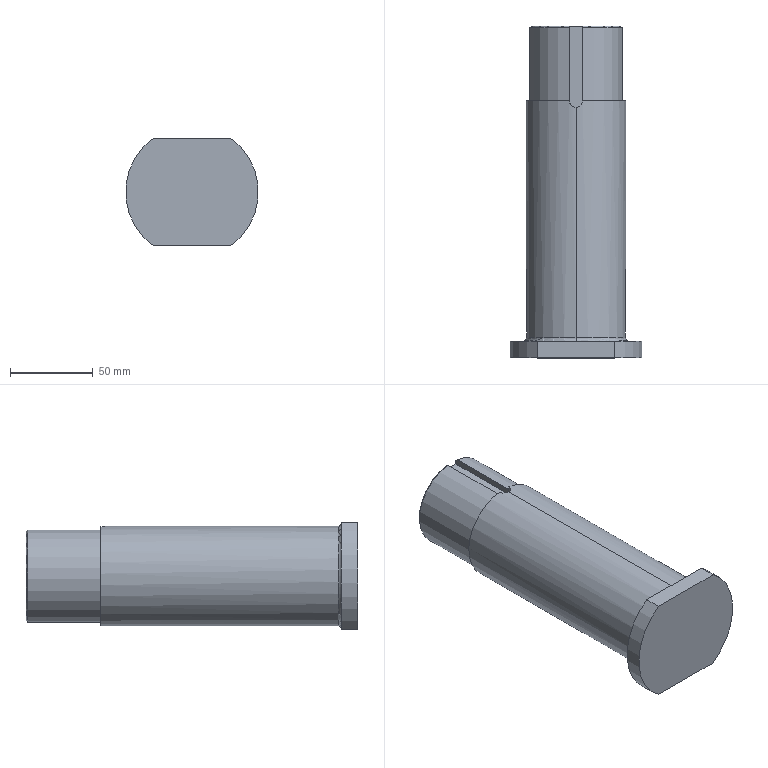Part | SolidWorks | features Fillet 2, ICE 2, Chamfer 1, Revolution 1 | 1 solid | 19 faces | box 80 x 200 x 65 mm | volume 564846 mm3 | plane 9 | cylinder 6 | torus 2 | cone 2 | commonest cylinder face diameters 60 x2 80 x2 8 x1 56 x1
STEP:
#1=CARTESIAN_POINT('',(0.,10.,32.));
#2=VERTEX_POINT('',#1);
#3=CARTESIAN_POINT('',(0.,10.,-32.));
#4=VERTEX_POINT('',#3);
#5=CARTESIAN_POINT('',(0.,10.,0.));
#6=DIRECTION('',(0.,-1.,0.));
#7=DIRECTION('',(0.,0.,-1.));
#8=AXIS2_PLACEMENT_3D('',#5,#6,#7);
#9=CIRCLE('',#8,32.);
#10=EDGE_CURVE('',#2,#4,#9,.T.);
#11=ORIENTED_EDGE('',*,*,#10,.F.);
#12=CARTESIAN_POINT('',(0.,12.,30.));
#13=VERTEX_POINT('',#12);
#14=CARTESIAN_POINT('',(0.,12.,32.));
#15=DIRECTION('',(1.,0.,0.));
#16=DIRECTION('',(0.,0.,-1.));
#17=AXIS2_PLACEMENT_3D('',#14,#15,#16);
#18=CIRCLE('',#17,2.);
#19=EDGE_CURVE('',#2,#13,#18,.T.);
#20=ORIENTED_EDGE('',*,*,#19,.T.);
#21=CARTESIAN_POINT('',(0.,12.,-30.));
#22=VERTEX_POINT('',#21);
#23=CARTESIAN_POINT('',(0.,12.,0.));
#24=DIRECTION('',(0.,1.,0.));
#25=DIRECTION('',(0.,0.,-1.));
#26=AXIS2_PLACEMENT_3D('',#23,#24,#25);
#27=CIRCLE('',#26,30.);
#28=EDGE_CURVE('',#22,#13,#27,.T.);
#29=ORIENTED_EDGE('',*,*,#28,.F.);
#30=CARTESIAN_POINT('',(0.,12.,-32.));
#31=DIRECTION('',(-1.,0.,0.));
#32=DIRECTION('',(0.,0.,1.));
#33=AXIS2_PLACEMENT_3D('',#30,#31,#32);
#34=CIRCLE('',#33,2.);
#35=EDGE_CURVE('',#4,#22,#34,.T.);
#36=ORIENTED_EDGE('',*,*,#35,.F.);
#37=EDGE_LOOP('',(#11,#20,#29,#36));
#38=FACE_OUTER_BOUND('',#37,.T.);
#39=CARTESIAN_POINT('',(0.,12.,0.));
#40=DIRECTION('',(0.,-1.,0.));
#41=DIRECTION('',(0.,0.,-1.));
#42=AXIS2_PLACEMENT_3D('',#39,#40,#41);
#43=TOROIDAL_SURFACE('',#42,32.,2.);
#44=ADVANCED_FACE('',(#38),#43,.F.);
#45=CARTESIAN_POINT('',(0.,200.,-27.));
#46=VERTEX_POINT('',#45);
#47=CARTESIAN_POINT('',(-4.,200.,26.702));
#48=VERTEX_POINT('',#47);
#49=CARTESIAN_POINT('',(0.,200.,0.));
#50=DIRECTION('',(0.,1.,0.));
#51=DIRECTION('',(0.,0.,-1.));
#52=AXIS2_PLACEMENT_3D('',#49,#50,#51);
#53=CIRCLE('',#52,27.);
#54=EDGE_CURVE('',#46,#48,#53,.T.);
#55=ORIENTED_EDGE('',*,*,#54,.F.);
#56=CARTESIAN_POINT('',(0.,199.,-28.));
#57=VERTEX_POINT('',#56);
#58=CARTESIAN_POINT('',(0.,200.,-27.));
#59=DIRECTION('',(0.,-0.7071,-0.7071));
#60=VECTOR('',#59,1000.);
#61=LINE('',#58,#60);
#62=EDGE_CURVE('',#46,#57,#61,.T.);
#63=ORIENTED_EDGE('',*,*,#62,.T.);
#64=CARTESIAN_POINT('',(-4.,199.,27.713));
#65=VERTEX_POINT('',#64);
#66=CARTESIAN_POINT('',(0.,199.,0.));
#67=DIRECTION('',(0.,-1.,0.));
#68=DIRECTION('',(0.,0.,-1.));
#69=AXIS2_PLACEMENT_3D('',#66,#67,#68);
#70=CIRCLE('',#69,28.);
#71=EDGE_CURVE('',#65,#57,#70,.T.);
#72=ORIENTED_EDGE('',*,*,#71,.F.);
#73=CARTESIAN_POINT('',(-4.,200.,26.702));
#74=CARTESIAN_POINT('',(-4.,199.667,27.039));
#75=CARTESIAN_POINT('',(-4.,199.333,27.376));
#76=CARTESIAN_POINT('',(-4.,199.,27.713));
#77=B_SPLINE_CURVE_WITH_KNOTS('',3,(#73,#74,#75,#76),.UNSPECIFIED.,.F.,.F.,(4,4),(0.,0.001422),.UNSPECIFIED.);
#78=EDGE_CURVE('',#48,#65,#77,.T.);
#79=ORIENTED_EDGE('',*,*,#78,.F.);
#80=EDGE_LOOP('',(#55,#63,#72,#79));
#81=FACE_OUTER_BOUND('',#80,.T.);
#82=CARTESIAN_POINT('',(0.,200.,0.));
#83=DIRECTION('',(0.,-1.,0.));
#84=DIRECTION('',(0.,0.,-1.));
#85=AXIS2_PLACEMENT_3D('',#82,#83,#84);
#86=CONICAL_SURFACE('',#85,27.,0.7854);
#87=ADVANCED_FACE('',(#81),#86,.T.);
#88=CARTESIAN_POINT('',(0.,12.,0.));
#89=DIRECTION('',(0.,1.,0.));
#90=DIRECTION('',(0.,0.,-1.));
#91=AXIS2_PLACEMENT_3D('',#88,#89,#90);
#92=CIRCLE('',#91,30.);
#93=EDGE_CURVE('',#13,#22,#92,.T.);
#94=ORIENTED_EDGE('',*,*,#93,.T.);
#95=CARTESIAN_POINT('',(0.,155.,-30.));
#96=VERTEX_POINT('',#95);
#97=CARTESIAN_POINT('',(0.,0.,-30.));
#98=DIRECTION('',(0.,1.,0.));
#99=VECTOR('',#98,1000.);
#100=LINE('',#97,#99);
#101=EDGE_CURVE('',#22,#96,#100,.T.);
#102=ORIENTED_EDGE('',*,*,#101,.T.);
#103=CARTESIAN_POINT('',(4.,155.,29.732));
#104=VERTEX_POINT('',#103);
#105=CARTESIAN_POINT('',(0.,155.,0.));
#106=DIRECTION('',(0.,1.,0.));
#107=DIRECTION('',(0.,0.,1.));
#108=AXIS2_PLACEMENT_3D('',#105,#106,#107);
#109=CIRCLE('',#108,30.);
#110=EDGE_CURVE('',#104,#96,#109,.T.);
#111=ORIENTED_EDGE('',*,*,#110,.F.);
#112=CARTESIAN_POINT('',(0.,151.,30.));
#113=VERTEX_POINT('',#112);
#114=CARTESIAN_POINT('',(4.,155.,29.732));
#115=CARTESIAN_POINT('',(4.,154.735,29.732));
#116=CARTESIAN_POINT('',(3.974,154.475,29.736));
#117=CARTESIAN_POINT('',(3.872,153.963,29.749));
#118=CARTESIAN_POINT('',(3.795,153.709,29.759));
#119=CARTESIAN_POINT('',(3.594,153.225,29.784));
#120=CARTESIAN_POINT('',(3.471,152.995,29.799));
#121=CARTESIAN_POINT('',(3.181,152.56,29.831));
#122=CARTESIAN_POINT('',(3.012,152.355,29.849));
#123=CARTESIAN_POINT('',(2.643,151.986,29.884));
#124=CARTESIAN_POINT('',(2.442,151.821,29.901));
#125=CARTESIAN_POINT('',(2.004,151.528,29.934));
#126=CARTESIAN_POINT('',(1.772,151.404,29.949));
#127=CARTESIAN_POINT('',(1.29,151.205,29.973));
#128=CARTESIAN_POINT('',(1.038,151.128,29.983));
#129=CARTESIAN_POINT('',(0.5211,151.025,29.997));
#130=CARTESIAN_POINT('',(0.2613,151.,30.));
#131=CARTESIAN_POINT('',(0.,151.,30.));
#132=B_SPLINE_CURVE_WITH_KNOTS('',3,(#114,#115,#116,#117,#118,#119,#120,#121,#122,#123,#124,#125,#126,#127,#128,#129,#130,#131),.UNSPECIFIED.,.F.,.F.,(4,2,2,2,2,2,2,2,4),(0.,0.0007827,0.001565,0.002348,0.003131,0.003913,0.004696,0.005479,0.006261),.UNSPECIFIED.);
#133=EDGE_CURVE('',#104,#113,#132,.T.);
#134=ORIENTED_EDGE('',*,*,#133,.T.);
#135=CARTESIAN_POINT('',(0.,0.,30.));
#136=DIRECTION('',(0.,1.,0.));
#137=VECTOR('',#136,1000.);
#138=LINE('',#135,#137);
#139=EDGE_CURVE('',#13,#113,#138,.T.);
#140=ORIENTED_EDGE('',*,*,#139,.F.);
#141=EDGE_LOOP('',(#94,#102,#111,#134,#140));
#142=FACE_OUTER_BOUND('',#141,.T.);
#143=CARTESIAN_POINT('',(0.,0.,0.));
#144=DIRECTION('',(0.,1.,0.));
#145=DIRECTION('',(0.,0.,1.));
#146=AXIS2_PLACEMENT_3D('',#143,#144,#145);
#147=CYLINDRICAL_SURFACE('',#146,30.);
#148=ADVANCED_FACE('',(#142),#147,.T.);
#149=ORIENTED_EDGE('',*,*,#101,.F.);
#150=ORIENTED_EDGE('',*,*,#28,.T.);
#151=ORIENTED_EDGE('',*,*,#139,.T.);
#152=CARTESIAN_POINT('',(-4.,155.,29.732));
#153=VERTEX_POINT('',#152);
#154=CARTESIAN_POINT('',(0.,151.,30.));
#155=CARTESIAN_POINT('',(-0.261,151.,30.));
#156=CARTESIAN_POINT('',(-0.5262,151.026,29.996));
#157=CARTESIAN_POINT('',(-1.039,151.128,29.983));
#158=CARTESIAN_POINT('',(-1.288,151.204,29.973));
#159=CARTESIAN_POINT('',(-1.773,151.405,29.949));
#160=CARTESIAN_POINT('',(-2.006,151.53,29.934));
#161=CARTESIAN_POINT('',(-2.439,151.819,29.901));
#162=CARTESIAN_POINT('',(-2.641,151.984,29.884));
#163=CARTESIAN_POINT('',(-3.014,152.357,29.849));
#164=CARTESIAN_POINT('',(-3.179,152.559,29.831));
#165=CARTESIAN_POINT('',(-3.469,152.991,29.799));
#166=CARTESIAN_POINT('',(-3.594,153.225,29.784));
#167=CARTESIAN_POINT('',(-3.795,153.709,29.759));
#168=CARTESIAN_POINT('',(-3.871,153.958,29.749));
#169=CARTESIAN_POINT('',(-3.973,154.471,29.736));
#170=CARTESIAN_POINT('',(-4.,154.736,29.732));
#171=CARTESIAN_POINT('',(-4.,155.,29.732));
#172=B_SPLINE_CURVE_WITH_KNOTS('',3,(#154,#155,#156,#157,#158,#159,#160,#161,#162,#163,#164,#165,#166,#167,#168,#169,#170,#171),.UNSPECIFIED.,.F.,.F.,(4,2,2,2,2,2,2,2,4),(0.006261,0.007043,0.007825,0.008607,0.009389,0.01017,0.01095,0.01173,0.01252),.UNSPECIFIED.);
#173=EDGE_CURVE('',#113,#153,#172,.T.);
#174=ORIENTED_EDGE('',*,*,#173,.T.);
#175=CARTESIAN_POINT('',(0.,155.,0.));
#176=DIRECTION('',(0.,1.,0.));
#177=DIRECTION('',(0.,0.,1.));
#178=AXIS2_PLACEMENT_3D('',#175,#176,#177);
#179=CIRCLE('',#178,30.);
#180=EDGE_CURVE('',#96,#153,#179,.T.);
#181=ORIENTED_EDGE('',*,*,#180,.F.);
#182=EDGE_LOOP('',(#149,#150,#151,#174,#181));
#183=FACE_OUTER_BOUND('',#182,.T.);
#184=CARTESIAN_POINT('',(0.,0.,0.));
#185=DIRECTION('',(0.,1.,0.));
#186=DIRECTION('',(0.,0.,1.));
#187=AXIS2_PLACEMENT_3D('',#184,#185,#186);
#188=CYLINDRICAL_SURFACE('',#187,30.);
#189=ADVANCED_FACE('',(#183),#188,.T.);
#190=CARTESIAN_POINT('',(-4.,155.,27.713));
#191=VERTEX_POINT('',#190);
#192=CARTESIAN_POINT('',(-4.,155.,32.501));
#193=DIRECTION('',(0.,0.,-1.));
#194=VECTOR('',#193,1000.);
#195=LINE('',#192,#194);
#196=EDGE_CURVE('',#153,#191,#195,.T.);
#197=ORIENTED_EDGE('',*,*,#196,.T.);
#198=CARTESIAN_POINT('',(4.,155.,27.713));
#199=VERTEX_POINT('',#198);
#200=CARTESIAN_POINT('',(0.,155.,0.));
#201=DIRECTION('',(0.,1.,0.));
#202=DIRECTION('',(0.,0.,1.));
#203=AXIS2_PLACEMENT_3D('',#200,#201,#202);
#204=CIRCLE('',#203,28.);
#205=EDGE_CURVE('',#199,#191,#204,.T.);
#206=ORIENTED_EDGE('',*,*,#205,.F.);
#207=CARTESIAN_POINT('',(4.,155.,32.501));
#208=DIRECTION('',(0.,0.,-1.));
#209=VECTOR('',#208,1000.);
#210=LINE('',#207,#209);
#211=EDGE_CURVE('',#104,#199,#210,.T.);
#212=ORIENTED_EDGE('',*,*,#211,.F.);
#213=ORIENTED_EDGE('',*,*,#110,.T.);
#214=ORIENTED_EDGE('',*,*,#180,.T.);
#215=EDGE_LOOP('',(#197,#206,#212,#213,#214));
#216=FACE_OUTER_BOUND('',#215,.T.);
#217=CARTESIAN_POINT('',(30.,155.,0.));
#218=DIRECTION('',(0.,-1.,0.));
#219=DIRECTION('',(0.,0.,-1.));
#220=AXIS2_PLACEMENT_3D('',#217,#218,#219);
#221=PLANE('',#220);
#222=ADVANCED_FACE('',(#216),#221,.F.);
#223=CARTESIAN_POINT('',(-4.,0.,27.713));
#224=DIRECTION('',(0.,1.,0.));
#225=VECTOR('',#224,1000.);
#226=LINE('',#223,#225);
#227=EDGE_CURVE('',#191,#65,#226,.T.);
#228=ORIENTED_EDGE('',*,*,#227,.T.);
#229=ORIENTED_EDGE('',*,*,#71,.T.);
#230=CARTESIAN_POINT('',(4.,199.,27.713));
#231=VERTEX_POINT('',#230);
#232=CARTESIAN_POINT('',(0.,199.,0.));
#233=DIRECTION('',(0.,-1.,0.));
#234=DIRECTION('',(0.,0.,-1.));
#235=AXIS2_PLACEMENT_3D('',#232,#233,#234);
#236=CIRCLE('',#235,28.);
#237=EDGE_CURVE('',#57,#231,#236,.T.);
#238=ORIENTED_EDGE('',*,*,#237,.T.);
#239=CARTESIAN_POINT('',(4.,0.,27.713));
#240=DIRECTION('',(0.,-1.,0.));
#241=VECTOR('',#240,1000.);
#242=LINE('',#239,#241);
#243=EDGE_CURVE('',#231,#199,#242,.T.);
#244=ORIENTED_EDGE('',*,*,#243,.T.);
#245=ORIENTED_EDGE('',*,*,#205,.T.);
#246=EDGE_LOOP('',(#228,#229,#238,#244,#245));
#247=FACE_OUTER_BOUND('',#246,.T.);
#248=CARTESIAN_POINT('',(0.,0.,0.));
#249=DIRECTION('',(0.,1.,0.));
#250=DIRECTION('',(0.,0.,1.));
#251=AXIS2_PLACEMENT_3D('',#248,#249,#250);
#252=CYLINDRICAL_SURFACE('',#251,28.);
#253=ADVANCED_FACE('',(#247),#252,.T.);
#254=CARTESIAN_POINT('',(4.,200.,24.));
#255=VERTEX_POINT('',#254);
#256=CARTESIAN_POINT('',(4.,200.,26.702));
#257=VERTEX_POINT('',#256);
#258=CARTESIAN_POINT('',(4.,200.,32.501));
#259=DIRECTION('',(0.,0.,1.));
#260=VECTOR('',#259,1000.);
#261=LINE('',#258,#260);
#262=EDGE_CURVE('',#255,#257,#261,.T.);
#263=ORIENTED_EDGE('',*,*,#262,.T.);
#264=CARTESIAN_POINT('',(0.,200.,0.));
#265=DIRECTION('',(0.,1.,0.));
#266=DIRECTION('',(0.,0.,-1.));
#267=AXIS2_PLACEMENT_3D('',#264,#265,#266);
#268=CIRCLE('',#267,27.);
#269=EDGE_CURVE('',#257,#46,#268,.T.);
#270=ORIENTED_EDGE('',*,*,#269,.T.);
#271=ORIENTED_EDGE('',*,*,#54,.T.);
#272=CARTESIAN_POINT('',(-4.,200.,24.));
#273=VERTEX_POINT('',#272);
#274=CARTESIAN_POINT('',(-4.,200.,32.501));
#275=DIRECTION('',(0.,0.,-1.));
#276=VECTOR('',#275,1000.);
#277=LINE('',#274,#276);
#278=EDGE_CURVE('',#48,#273,#277,.T.);
#279=ORIENTED_EDGE('',*,*,#278,.T.);
#280=CARTESIAN_POINT('',(0.,200.,24.));
#281=DIRECTION('',(1.,0.,0.));
#282=VECTOR('',#281,1000.);
#283=LINE('',#280,#282);
#284=EDGE_CURVE('',#273,#255,#283,.T.);
#285=ORIENTED_EDGE('',*,*,#284,.T.);
#286=EDGE_LOOP('',(#263,#270,#271,#279,#285));
#287=FACE_OUTER_BOUND('',#286,.T.);
#288=CARTESIAN_POINT('',(28.,200.,0.));
#289=DIRECTION('',(0.,-1.,0.));
#290=DIRECTION('',(0.,0.,-1.));
#291=AXIS2_PLACEMENT_3D('',#288,#289,#290);
#292=PLANE('',#291);
#293=ADVANCED_FACE('',(#287),#292,.F.);
#294=CARTESIAN_POINT('',(-23.318,0.,-32.5));
#295=VERTEX_POINT('',#294);
#296=CARTESIAN_POINT('',(-23.318,0.,32.5));
#297=VERTEX_POINT('',#296);
#298=CARTESIAN_POINT('',(0.,0.,0.));
#299=DIRECTION('',(0.,1.,0.));
#300=DIRECTION('',(0.,0.,1.));
#301=AXIS2_PLACEMENT_3D('',#298,#299,#300);
#302=CIRCLE('',#301,40.);
#303=EDGE_CURVE('',#295,#297,#302,.T.);
#304=ORIENTED_EDGE('',*,*,#303,.T.);
#305=CARTESIAN_POINT('',(-23.318,10.,32.5));
#306=VERTEX_POINT('',#305);
#307=CARTESIAN_POINT('',(-23.318,0.,32.5));
#308=DIRECTION('',(0.,1.,0.));
#309=VECTOR('',#308,1000.);
#310=LINE('',#307,#309);
#311=EDGE_CURVE('',#297,#306,#310,.T.);
#312=ORIENTED_EDGE('',*,*,#311,.T.);
#313=CARTESIAN_POINT('',(-23.318,10.,-32.5));
#314=VERTEX_POINT('',#313);
#315=CARTESIAN_POINT('',(0.,10.,0.));
#316=DIRECTION('',(0.,1.,0.));
#317=DIRECTION('',(0.,0.,1.));
#318=AXIS2_PLACEMENT_3D('',#315,#316,#317);
#319=CIRCLE('',#318,40.);
#320=EDGE_CURVE('',#314,#306,#319,.T.);
#321=ORIENTED_EDGE('',*,*,#320,.F.);
#322=CARTESIAN_POINT('',(-23.318,0.,-32.5));
#323=DIRECTION('',(0.,-1.,0.));
#324=VECTOR('',#323,1000.);
#325=LINE('',#322,#324);
#326=EDGE_CURVE('',#314,#295,#325,.T.);
#327=ORIENTED_EDGE('',*,*,#326,.T.);
#328=EDGE_LOOP('',(#304,#312,#321,#327));
#329=FACE_OUTER_BOUND('',#328,.T.);
#330=CARTESIAN_POINT('',(0.,0.,0.));
#331=DIRECTION('',(0.,1.,0.));
#332=DIRECTION('',(0.,0.,1.));
#333=AXIS2_PLACEMENT_3D('',#330,#331,#332);
#334=CYLINDRICAL_SURFACE('',#333,40.);
#335=ADVANCED_FACE('',(#329),#334,.T.);
#336=CARTESIAN_POINT('',(23.318,0.,32.5));
#337=VERTEX_POINT('',#336);
#338=CARTESIAN_POINT('',(23.318,0.,-32.5));
#339=VERTEX_POINT('',#338);
#340=CARTESIAN_POINT('',(0.,0.,0.));
#341=DIRECTION('',(0.,1.,0.));
#342=DIRECTION('',(0.,0.,1.));
#343=AXIS2_PLACEMENT_3D('',#340,#341,#342);
#344=CIRCLE('',#343,40.);
#345=EDGE_CURVE('',#337,#339,#344,.T.);
#346=ORIENTED_EDGE('',*,*,#345,.F.);
#347=CARTESIAN_POINT('',(65.,0.,32.5));
#348=DIRECTION('',(1.,0.,0.));
#349=VECTOR('',#348,1000.);
#350=LINE('',#347,#349);
#351=EDGE_CURVE('',#297,#337,#350,.T.);
#352=ORIENTED_EDGE('',*,*,#351,.F.);
#353=ORIENTED_EDGE('',*,*,#303,.F.);
#354=CARTESIAN_POINT('',(65.,0.,-32.5));
#355=DIRECTION('',(-1.,0.,0.));
#356=VECTOR('',#355,1000.);
#357=LINE('',#354,#356);
#358=EDGE_CURVE('',#339,#295,#357,.T.);
#359=ORIENTED_EDGE('',*,*,#358,.F.);
#360=EDGE_LOOP('',(#346,#352,#353,#359));
#361=FACE_OUTER_BOUND('',#360,.T.);
#362=CARTESIAN_POINT('',(0.,0.,0.));
#363=DIRECTION('',(0.,1.,0.));
#364=DIRECTION('',(0.,0.,1.));
#365=AXIS2_PLACEMENT_3D('',#362,#363,#364);
#366=PLANE('',#365);
#367=ADVANCED_FACE('',(#361),#366,.F.);
#368=CARTESIAN_POINT('',(23.318,10.,32.5));
#369=VERTEX_POINT('',#368);
#370=CARTESIAN_POINT('',(23.318,10.,-32.5));
#371=VERTEX_POINT('',#370);
#372=CARTESIAN_POINT('',(0.,10.,0.));
#373=DIRECTION('',(0.,1.,0.));
#374=DIRECTION('',(0.,0.,1.));
#375=AXIS2_PLACEMENT_3D('',#372,#373,#374);
#376=CIRCLE('',#375,40.);
#377=EDGE_CURVE('',#369,#371,#376,.T.);
#378=ORIENTED_EDGE('',*,*,#377,.F.);
#379=CARTESIAN_POINT('',(23.318,0.,32.5));
#380=DIRECTION('',(0.,-1.,0.));
#381=VECTOR('',#380,1000.);
#382=LINE('',#379,#381);
#383=EDGE_CURVE('',#369,#337,#382,.T.);
#384=ORIENTED_EDGE('',*,*,#383,.T.);
#385=ORIENTED_EDGE('',*,*,#345,.T.);
#386=CARTESIAN_POINT('',(23.318,0.,-32.5));
#387=DIRECTION('',(0.,1.,0.));
#388=VECTOR('',#387,1000.);
#389=LINE('',#386,#388);
#390=EDGE_CURVE('',#339,#371,#389,.T.);
#391=ORIENTED_EDGE('',*,*,#390,.T.);
#392=EDGE_LOOP('',(#378,#384,#385,#391));
#393=FACE_OUTER_BOUND('',#392,.T.);
#394=CARTESIAN_POINT('',(0.,0.,0.));
#395=DIRECTION('',(0.,1.,0.));
#396=DIRECTION('',(0.,0.,1.));
#397=AXIS2_PLACEMENT_3D('',#394,#395,#396);
#398=CYLINDRICAL_SURFACE('',#397,40.);
#399=ADVANCED_FACE('',(#393),#398,.T.);
#400=CARTESIAN_POINT('',(0.,10.,0.));
#401=DIRECTION('',(0.,-1.,0.));
#402=DIRECTION('',(0.,0.,-1.));
#403=AXIS2_PLACEMENT_3D('',#400,#401,#402);
#404=CIRCLE('',#403,32.);
#405=EDGE_CURVE('',#4,#2,#404,.T.);
#406=ORIENTED_EDGE('',*,*,#405,.T.);
#407=ORIENTED_EDGE('',*,*,#10,.T.);
#408=EDGE_LOOP('',(#406,#407));
#409=FACE_BOUND('',#408,.T.);
#410=ORIENTED_EDGE('',*,*,#320,.T.);
#411=CARTESIAN_POINT('',(40.,10.,32.5));
#412=DIRECTION('',(1.,0.,0.));
#413=VECTOR('',#412,1000.);
#414=LINE('',#411,#413);
#415=EDGE_CURVE('',#306,#369,#414,.T.);
#416=ORIENTED_EDGE('',*,*,#415,.T.);
#417=ORIENTED_EDGE('',*,*,#377,.T.);
#418=CARTESIAN_POINT('',(40.,10.,-32.5));
#419=DIRECTION('',(-1.,0.,0.));
#420=VECTOR('',#419,1000.);
#421=LINE('',#418,#420);
#422=EDGE_CURVE('',#371,#314,#421,.T.);
#423=ORIENTED_EDGE('',*,*,#422,.T.);
#424=EDGE_LOOP('',(#410,#416,#417,#423));
#425=FACE_OUTER_BOUND('',#424,.T.);
#426=CARTESIAN_POINT('',(40.,10.,0.));
#427=DIRECTION('',(0.,-1.,0.));
#428=DIRECTION('',(0.,0.,-1.));
#429=AXIS2_PLACEMENT_3D('',#426,#427,#428);
#430=PLANE('',#429);
#431=ADVANCED_FACE('',(#409,#425),#430,.F.);
#432=ORIENTED_EDGE('',*,*,#358,.T.);
#433=ORIENTED_EDGE('',*,*,#326,.F.);
#434=ORIENTED_EDGE('',*,*,#422,.F.);
#435=ORIENTED_EDGE('',*,*,#390,.F.);
#436=EDGE_LOOP('',(#432,#433,#434,#435));
#437=FACE_OUTER_BOUND('',#436,.T.);
#438=CARTESIAN_POINT('',(65.,10.,-32.5));
#439=DIRECTION('',(0.,0.,1.));
#440=DIRECTION('',(1.,0.,0.));
#441=AXIS2_PLACEMENT_3D('',#438,#439,#440);
#442=PLANE('',#441);
#443=ADVANCED_FACE('',(#437),#442,.F.);
#444=ORIENTED_EDGE('',*,*,#351,.T.);
#445=ORIENTED_EDGE('',*,*,#383,.F.);
#446=ORIENTED_EDGE('',*,*,#415,.F.);
#447=ORIENTED_EDGE('',*,*,#311,.F.);
#448=EDGE_LOOP('',(#444,#445,#446,#447));
#449=FACE_OUTER_BOUND('',#448,.T.);
#450=CARTESIAN_POINT('',(65.,10.,32.5));
#451=DIRECTION('',(0.,0.,-1.));
#452=DIRECTION('',(-1.,0.,0.));
#453=AXIS2_PLACEMENT_3D('',#450,#451,#452);
#454=PLANE('',#453);
#455=ADVANCED_FACE('',(#449),#454,.F.);
#456=ORIENTED_EDGE('',*,*,#278,.F.);
#457=ORIENTED_EDGE('',*,*,#78,.T.);
#458=ORIENTED_EDGE('',*,*,#227,.F.);
#459=CARTESIAN_POINT('',(-4.,155.,24.));
#460=VERTEX_POINT('',#459);
#461=CARTESIAN_POINT('',(-4.,155.,32.501));
#462=DIRECTION('',(0.,0.,-1.));
#463=VECTOR('',#462,1000.);
#464=LINE('',#461,#463);
#465=EDGE_CURVE('',#191,#460,#464,.T.);
#466=ORIENTED_EDGE('',*,*,#465,.T.);
#467=CARTESIAN_POINT('',(-4.,200.,24.));
#468=DIRECTION('',(0.,-1.,0.));
#469=VECTOR('',#468,1000.);
#470=LINE('',#467,#469);
#471=EDGE_CURVE('',#273,#460,#470,.T.);
#472=ORIENTED_EDGE('',*,*,#471,.F.);
#473=EDGE_LOOP('',(#456,#457,#458,#466,#472));
#474=FACE_OUTER_BOUND('',#473,.T.);
#475=CARTESIAN_POINT('',(-4.,200.,32.501));
#476=DIRECTION('',(1.,0.,0.));
#477=DIRECTION('',(0.,1.,0.));
#478=AXIS2_PLACEMENT_3D('',#475,#476,#477);
#479=PLANE('',#478);
#480=ADVANCED_FACE('',(#474),#479,.T.);
#481=ORIENTED_EDGE('',*,*,#211,.T.);
#482=CARTESIAN_POINT('',(4.,155.,24.));
#483=VERTEX_POINT('',#482);
#484=CARTESIAN_POINT('',(4.,155.,32.501));
#485=DIRECTION('',(0.,0.,-1.));
#486=VECTOR('',#485,1000.);
#487=LINE('',#484,#486);
#488=EDGE_CURVE('',#199,#483,#487,.T.);
#489=ORIENTED_EDGE('',*,*,#488,.T.);
#490=CARTESIAN_POINT('',(0.,155.,24.));
#491=DIRECTION('',(0.,0.,1.));
#492=DIRECTION('',(1.,0.,0.));
#493=AXIS2_PLACEMENT_3D('',#490,#491,#492);
#494=CIRCLE('',#493,4.);
#495=EDGE_CURVE('',#460,#483,#494,.T.);
#496=ORIENTED_EDGE('',*,*,#495,.F.);
#497=ORIENTED_EDGE('',*,*,#465,.F.);
#498=ORIENTED_EDGE('',*,*,#196,.F.);
#499=ORIENTED_EDGE('',*,*,#173,.F.);
#500=ORIENTED_EDGE('',*,*,#133,.F.);
#501=EDGE_LOOP('',(#481,#489,#496,#497,#498,#499,#500));
#502=FACE_OUTER_BOUND('',#501,.T.);
#503=CARTESIAN_POINT('',(0.,155.,32.501));
#504=DIRECTION('',(0.,0.,-1.));
#505=DIRECTION('',(-1.,0.,0.));
#506=AXIS2_PLACEMENT_3D('',#503,#504,#505);
#507=CYLINDRICAL_SURFACE('',#506,4.);
#508=ADVANCED_FACE('',(#502),#507,.F.);
#509=ORIENTED_EDGE('',*,*,#243,.F.);
#510=CARTESIAN_POINT('',(4.,199.,27.713));
#511=CARTESIAN_POINT('',(4.,199.333,27.376));
#512=CARTESIAN_POINT('',(4.,199.667,27.039));
#513=CARTESIAN_POINT('',(4.,200.,26.702));
#514=B_SPLINE_CURVE_WITH_KNOTS('',3,(#510,#511,#512,#513),.UNSPECIFIED.,.F.,.F.,(4,4),(0.,0.001422),.UNSPECIFIED.);
#515=EDGE_CURVE('',#231,#257,#514,.T.);
#516=ORIENTED_EDGE('',*,*,#515,.T.);
#517=ORIENTED_EDGE('',*,*,#262,.F.);
#518=CARTESIAN_POINT('',(4.,200.,24.));
#519=DIRECTION('',(0.,1.,0.));
#520=VECTOR('',#519,1000.);
#521=LINE('',#518,#520);
#522=EDGE_CURVE('',#483,#255,#521,.T.);
#523=ORIENTED_EDGE('',*,*,#522,.F.);
#524=ORIENTED_EDGE('',*,*,#488,.F.);
#525=EDGE_LOOP('',(#509,#516,#517,#523,#524));
#526=FACE_OUTER_BOUND('',#525,.T.);
#527=CARTESIAN_POINT('',(4.,200.,32.501));
#528=DIRECTION('',(-1.,0.,0.));
#529=DIRECTION('',(0.,-1.,0.));
#530=AXIS2_PLACEMENT_3D('',#527,#528,#529);
#531=PLANE('',#530);
#532=ADVANCED_FACE('',(#526),#531,.T.);
#533=ORIENTED_EDGE('',*,*,#471,.T.);
#534=ORIENTED_EDGE('',*,*,#495,.T.);
#535=ORIENTED_EDGE('',*,*,#522,.T.);
#536=ORIENTED_EDGE('',*,*,#284,.F.);
#537=EDGE_LOOP('',(#533,#534,#535,#536));
#538=FACE_OUTER_BOUND('',#537,.T.);
#539=CARTESIAN_POINT('',(0.,200.,24.));
#540=DIRECTION('',(0.,0.,1.));
#541=DIRECTION('',(1.,0.,0.));
#542=AXIS2_PLACEMENT_3D('',#539,#540,#541);
#543=PLANE('',#542);
#544=ADVANCED_FACE('',(#538),#543,.T.);
#545=ORIENTED_EDGE('',*,*,#62,.F.);
#546=ORIENTED_EDGE('',*,*,#269,.F.);
#547=ORIENTED_EDGE('',*,*,#515,.F.);
#548=ORIENTED_EDGE('',*,*,#237,.F.);
#549=EDGE_LOOP('',(#545,#546,#547,#548));
#550=FACE_OUTER_BOUND('',#549,.T.);
#551=CARTESIAN_POINT('',(0.,200.,0.));
#552=DIRECTION('',(0.,-1.,0.));
#553=DIRECTION('',(0.,0.,-1.));
#554=AXIS2_PLACEMENT_3D('',#551,#552,#553);
#555=CONICAL_SURFACE('',#554,27.,0.7854);
#556=ADVANCED_FACE('',(#550),#555,.T.);
#557=ORIENTED_EDGE('',*,*,#19,.F.);
#558=ORIENTED_EDGE('',*,*,#405,.F.);
#559=ORIENTED_EDGE('',*,*,#35,.T.);
#560=ORIENTED_EDGE('',*,*,#93,.F.);
#561=EDGE_LOOP('',(#557,#558,#559,#560));
#562=FACE_OUTER_BOUND('',#561,.T.);
#563=CARTESIAN_POINT('',(0.,12.,0.));
#564=DIRECTION('',(0.,-1.,0.));
#565=DIRECTION('',(0.,0.,-1.));
#566=AXIS2_PLACEMENT_3D('',#563,#564,#565);
#567=TOROIDAL_SURFACE('',#566,32.,2.);
#568=ADVANCED_FACE('',(#562),#567,.F.);
#569=CLOSED_SHELL('',(#44,#87,#148,#189,#222,#253,#293,#335,#367,#399,#431,#443,#455,#480,#508,#532,#544,#556,#568));
#570=MANIFOLD_SOLID_BREP('',#569);
#571=CARTESIAN_POINT('',(0.,0.,0.));
#572=DIRECTION('',(0.,0.,1.));
#573=DIRECTION('',(1.,0.,0.));
#574=AXIS2_PLACEMENT_3D('',#571,#572,#573);
#575=(LENGTH_UNIT()NAMED_UNIT(*)SI_UNIT(.MILLI.,.METRE.));
#576=UNCERTAINTY_MEASURE_WITH_UNIT(LENGTH_MEASURE(0.00001),#575,'','');
#577=(NAMED_UNIT(*)PLANE_ANGLE_UNIT()SI_UNIT($,.RADIAN.));
#578=(NAMED_UNIT(*)SI_UNIT($,.STERADIAN.)SOLID_ANGLE_UNIT());
#579=(GEOMETRIC_REPRESENTATION_CONTEXT(3)GLOBAL_UNCERTAINTY_ASSIGNED_CONTEXT((#576))GLOBAL_UNIT_ASSIGNED_CONTEXT((#575,#577,#578))REPRESENTATION_CONTEXT('',''));
#580=ADVANCED_BREP_SHAPE_REPRESENTATION('',(#570,#574),#579);